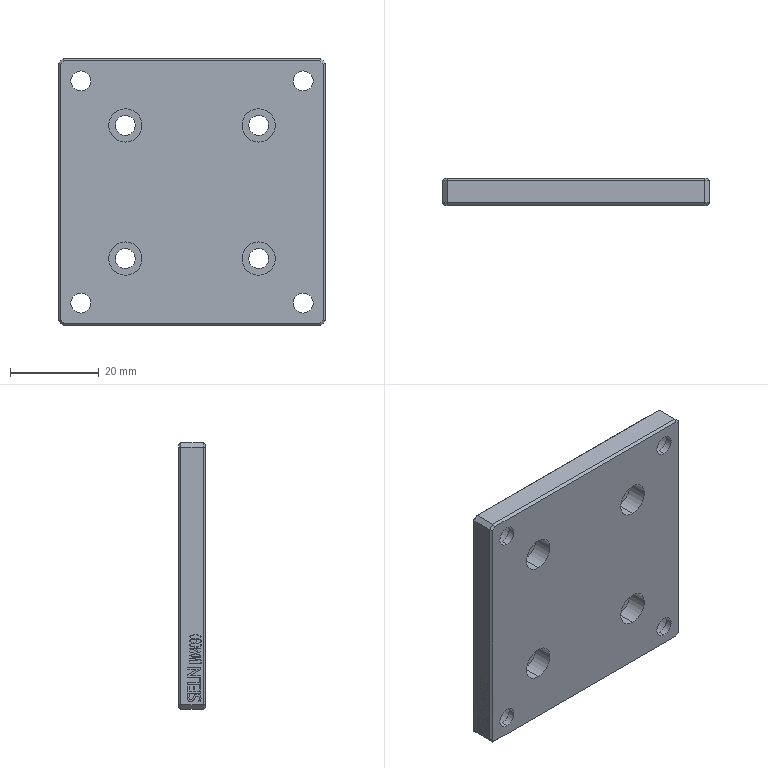Part | STEP file | Guide wheel mechanism revised.sldasm-Part-378 | 1 solid | 284 faces | box 60 x 6 x 60 mm | volume 19638 mm3 | plane 236 | cylinder 32 | spline 16 | commonest cylinder face diameters 4.5 x16 7.5 x8 8 x8